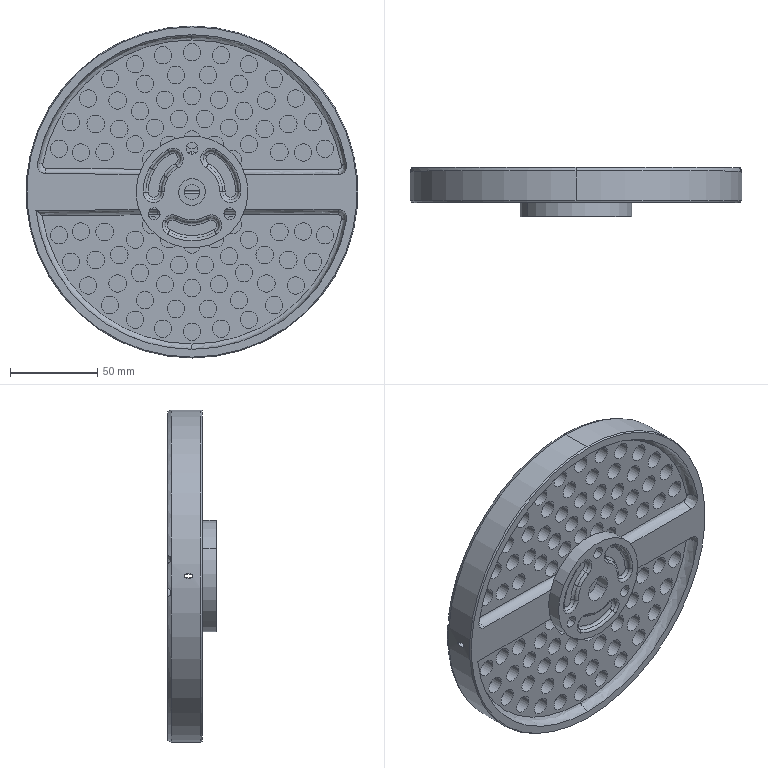Part | NX | features BREP 2 | 2 solids | 409 faces | box 190 x 28 x 190 mm | volume 281154 mm3 | cylinder 202 | plane 108 | spline 53 | torus 40 | cone 6 | commonest cylinder face diameters 10 x172 4.175 x6 6.8 x6 3.722 x2 5.496 x2 9 x2